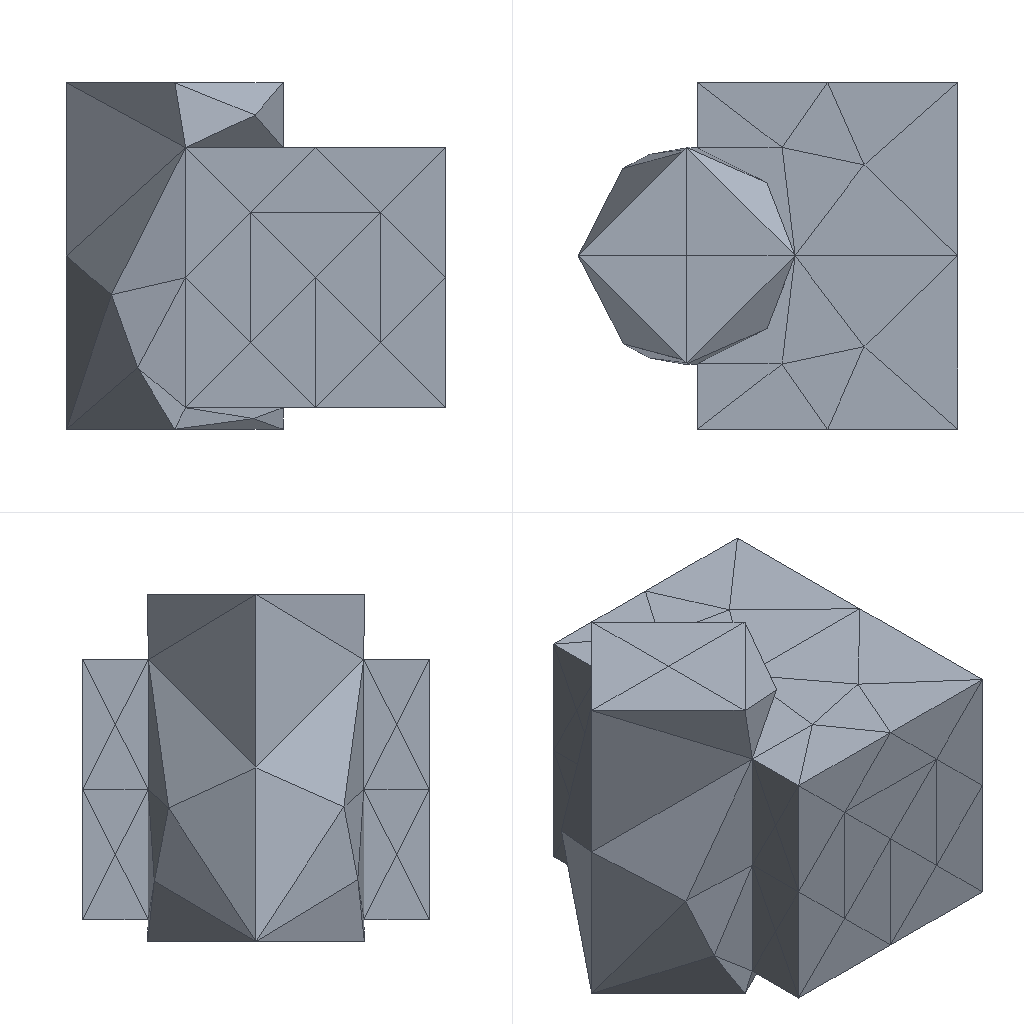Simulation study | ansys mapdl
Set-up summary:
category,name,step,type,value,unit,region
solver,ansys_mapdl
units,mm-N-s-tonne (MPa),,inferred,E=210000 density=
analysis,model,,static
mesh,nodes,,,434
mesh,elements,,,208
element_type,SOLID187,,,208
material,mat 1,,E,210000
material,mat 1,,nu,0.3
load,,model,body load temp,,,all
load,,model,force,"1000 [dir=(0, 0, -1) n=80]",,node list
bc,,model,fixed,"[dofs=UX,UY,UZ n=559]",,node list
Ansys APDL input file, long lists of numbers shortened:
/COM,ANSYS RELEASE 2026 R1           BUILD 26.1      UP20260202       09:08:10
/PREP7
/NOPR
/TITLE,2
ANTYPE, 0
*IF,_CDRDOFF,EQ,1,THEN     !if solid model was read in
_CDRDOFF=             !reset flag, numoffs already performed
*ELSE              !offset database for the following FE model
NUMOFF,NODE,      434
NUMOFF,ELEM,      208
NUMOFF,MAT ,        1
NUMOFF,TYPE,        1
*ENDIF
*SET,_RETURN ,  0.
*SET,_STATUS ,  0.
*SET,_UIQR   ,  80.
*SET,__FLOATPARAMETER__,  434.
DOF,DELETE
ETBLOCK,        1,        1
(2i9,19a9)
        1      187        0        0        0        0        0        0        0        0        0        0        0        0        0        0        0        0        0        0        0
       -1
NBLOCK,6,SOLID,       434,       434
(3i9,6e21.13e3)
        1        0        0 3.5500000000000E+001 6.1232339957368E-016-1.0000000000000E+000
! (433 more lines like these left out)
N,UNBL,LOC,       -1,
EBLOCK,19,SOLID,       208,       208
(19i10)
         1         1         1         1         0         0         0         0        10         0         1       279        14       280       281       287       288       289       290
! (415 more lines like these left out)
        -1
MPTEMP,UNBL, 1, 1,  0.    ,
MPDATA,UNBL, 1,EX  ,       1, 1,  210000.000    ,
MPTEMP,UNBL, 1, 1,  0.    ,
MPDATA,UNBL, 1,NUXY,       1, 1, 0.3    ,
MPTEMP,UNBL, 1, 1,  0.    ,
MPDATA,UNBL, 1,PRXY,       1, 1, 0.3    ,
EXTOPT,ATTR,      0,      0,      0
EXTOPT,ESIZE,  0,  0.
EXTOPT,ACLEAR,      0
TREF,  0.
IRLF,  0
BFUNIF,TEMP,_TINY
ACEL,  0.    ,  0.    ,  0.
OMEGA,  0.    ,  0.    ,  0.
DOMEGA,  0.    ,  0.    ,  0.
CGLOC,  0.    ,  0.    ,  0.
CGOMEGA,  0.    ,  0.    ,  0.
DCGOMG,  0.    ,  0.    ,  0.
KUSE,     0
TIME,  0.
ALPHAD,  0.
BETAD,  0.
DMPRAT,  0.
DMPSTR,  0.
CRPLIM, 0.1    ,   0
CRPLIM,  0.    ,   1
NCNV,     0, 1.000000000E+12,     0,  0.    ,  0.
NEQIT,     0
ERESX,DEFA
DBLOCK,       559
(i9,a6,2(pg16.9))
        1  UX    0.00000000      0.00000000
! (558 more lines like these left out)
       -1
FBLOCK,        80
(i9,a6,2(pg16.9))
       10  FZ   -12.5000000      0.00000000
! (79 more lines like these left out)
       -1
/GO
FINISH
Results summary:
result,analysis_type_db,,,static,unstated
result,n_sets,,,1,unstated
result,load_steps[0].set,load_step=1,,1,unstated
result,load_steps[0].substep,load_step=1,,1,unstated
result,load_steps[0].time,load_step=1,,1,unstated
result,load_steps[0].freq,load_step=1,,1,unstated
result,load_steps[0].max_usum,load_step=1,,0.0004697,unstated
result,load_steps[0].max_seqv,load_step=1,,17.458,unstated
result,load_steps[0].reaction_sum.FX,load_step=1,,4.11582e-12,unstated
result,load_steps[0].reaction_sum.FY,load_step=1,,8.47855e-12,unstated
result,load_steps[0].reaction_sum.FZ,load_step=1,,1000,unstated
result,load_steps[0].reaction_sum.MX,load_step=1,,0,unstated
result,load_steps[0].reaction_sum.MY,load_step=1,,0,unstated
result,load_steps[0].reaction_sum.MZ,load_step=1,,0,unstated
result,convergence,,,results present for all listed sets,unstated